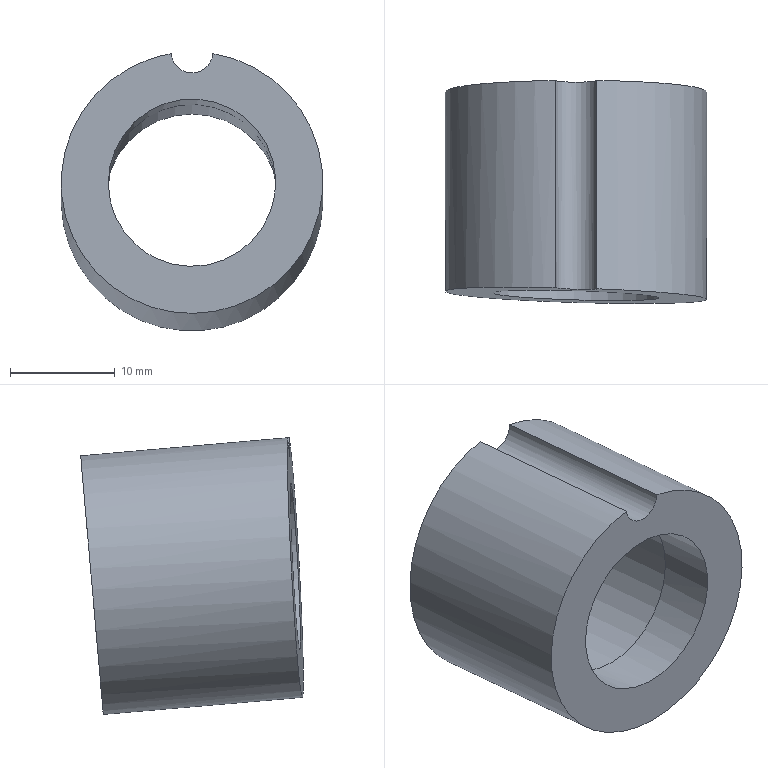Part | NX | features EKSD 25-20-16.00 2 | 1 solid | 7 faces | box 25 x 21.281 x 26.488 mm | volume 5318 mm3 | cylinder 4 | plane 3 | commonest cylinder face diameters 4 x1 16 x1 16.6 x1 25 x1
STEP:
#1=CARTESIAN_POINT('',(396.532,-42.364,-29.982));
#2=VERTEX_POINT('',#1);
#3=CARTESIAN_POINT('',(400.519,-42.364,-29.982));
#4=VERTEX_POINT('',#3);
#5=CARTESIAN_POINT('',(398.525,-42.35,-29.823));
#6=DIRECTION('',(0.,0.9962,-0.08716));
#7=DIRECTION('',(0.,0.08716,0.9962));
#8=AXIS2_PLACEMENT_3D('',#5,#6,#7);
#9=CIRCLE('',#8,2.);
#10=EDGE_CURVE('',#2,#4,#9,.F.);
#11=ORIENTED_EDGE('',*,*,#10,.T.);
#12=CARTESIAN_POINT('',(398.525,-43.44,-42.275));
#13=DIRECTION('',(0.,0.9962,-0.08716));
#14=DIRECTION('',(0.,0.08716,0.9962));
#15=AXIS2_PLACEMENT_3D('',#12,#13,#14);
#16=CIRCLE('',#15,12.5);
#17=EDGE_CURVE('',#2,#4,#16,.F.);
#18=ORIENTED_EDGE('',*,*,#17,.F.);
#19=EDGE_LOOP('',(#11,#18));
#20=FACE_BOUND('',#19,.T.);
#21=CARTESIAN_POINT('',(398.525,-42.717,-34.007));
#22=VERTEX_POINT('',#21);
#23=CARTESIAN_POINT('',(398.525,-43.44,-42.275));
#24=DIRECTION('',(0.,0.9962,-0.08716));
#25=DIRECTION('',(0.,0.08716,0.9962));
#26=AXIS2_PLACEMENT_3D('',#23,#24,#25);
#27=CIRCLE('',#26,8.3);
#28=EDGE_CURVE('',#22,#22,#27,.T.);
#29=ORIENTED_EDGE('',*,*,#28,.F.);
#30=EDGE_LOOP('',(#29));
#31=FACE_BOUND('',#30,.T.);
#32=CARTESIAN_POINT('',(398.525,-43.44,-42.275));
#33=DIRECTION('',(0.,0.9962,-0.08716));
#34=DIRECTION('',(0.,0.08716,0.9962));
#35=AXIS2_PLACEMENT_3D('',#32,#33,#34);
#36=PLANE('',#35);
#37=ADVANCED_FACE('',(#20,#31),#36,.T.);
#38=CARTESIAN_POINT('',(400.519,-62.276,-28.24));
#39=VERTEX_POINT('',#38);
#40=CARTESIAN_POINT('',(396.532,-62.155,-28.251));
#41=VERTEX_POINT('',#40);
#42=CARTESIAN_POINT('',(398.525,-62.207,-28.086));
#43=DIRECTION('',(0.03046,0.9981,-0.05344));
#44=DIRECTION('',(-0.6692,-0.01935,-0.7428));
#45=AXIS2_PLACEMENT_3D('',#42,#43,#44);
#46=ELLIPSE('',#45,2.002,2.);
#47=EDGE_CURVE('',#39,#41,#46,.T.);
#48=ORIENTED_EDGE('',*,*,#47,.T.);
#49=CARTESIAN_POINT('',(398.525,-62.876,-40.575));
#50=DIRECTION('',(0.03046,0.9981,-0.05344));
#51=DIRECTION('',(-0.6692,-0.01935,-0.7428));
#52=AXIS2_PLACEMENT_3D('',#49,#50,#51);
#53=ELLIPSE('',#52,12.513,12.5);
#54=EDGE_CURVE('',#39,#41,#53,.T.);
#55=ORIENTED_EDGE('',*,*,#54,.F.);
#56=EDGE_LOOP('',(#48,#55));
#57=FACE_BOUND('',#56,.T.);
#58=CARTESIAN_POINT('',(393.166,-63.031,-46.523));
#59=VERTEX_POINT('',#58);
#60=CARTESIAN_POINT('',(398.525,-62.876,-40.575));
#61=DIRECTION('',(0.03046,0.9981,-0.05344));
#62=DIRECTION('',(-0.6692,-0.01935,-0.7428));
#63=AXIS2_PLACEMENT_3D('',#60,#61,#62);
#64=ELLIPSE('',#63,8.008,8.);
#65=EDGE_CURVE('',#59,#59,#64,.F.);
#66=ORIENTED_EDGE('',*,*,#65,.F.);
#67=EDGE_LOOP('',(#66));
#68=FACE_BOUND('',#67,.T.);
#69=CARTESIAN_POINT('',(457.994,-68.531,-112.302));
#70=DIRECTION('',(0.03046,0.9981,-0.05344));
#71=DIRECTION('',(0.06614,0.05134,0.9965));
#72=AXIS2_PLACEMENT_3D('',#69,#70,#71);
#73=PLANE('',#72);
#74=ADVANCED_FACE('',(#57,#68),#73,.F.);
#75=CARTESIAN_POINT('',(400.519,-54.319,-28.936));
#76=DIRECTION('',(0.,0.9962,-0.08716));
#77=VECTOR('',#76,1000.);
#78=LINE('',#75,#77);
#79=EDGE_CURVE('',#39,#4,#78,.T.);
#80=ORIENTED_EDGE('',*,*,#79,.F.);
#81=ORIENTED_EDGE('',*,*,#54,.T.);
#82=CARTESIAN_POINT('',(396.532,-54.319,-28.936));
#83=DIRECTION('',(0.,0.9962,-0.08716));
#84=VECTOR('',#83,1000.);
#85=LINE('',#82,#84);
#86=EDGE_CURVE('',#2,#41,#85,.F.);
#87=ORIENTED_EDGE('',*,*,#86,.F.);
#88=ORIENTED_EDGE('',*,*,#17,.T.);
#89=EDGE_LOOP('',(#80,#81,#87,#88));
#90=FACE_BOUND('',#89,.T.);
#91=CARTESIAN_POINT('',(398.525,-65.356,-40.358));
#92=DIRECTION('',(0.,0.9962,-0.08716));
#93=DIRECTION('',(0.,0.08716,0.9962));
#94=AXIS2_PLACEMENT_3D('',#91,#92,#93);
#95=CYLINDRICAL_SURFACE('',#94,12.5);
#96=ADVANCED_FACE('',(#90),#95,.T.);
#97=CARTESIAN_POINT('',(398.525,-58.084,-49.025));
#98=VERTEX_POINT('',#97);
#99=CARTESIAN_POINT('',(398.525,-57.387,-41.055));
#100=DIRECTION('',(0.,-0.9962,0.08716));
#101=DIRECTION('',(0.,-0.08716,-0.9962));
#102=AXIS2_PLACEMENT_3D('',#99,#100,#101);
#103=CIRCLE('',#102,8.);
#104=EDGE_CURVE('',#98,#98,#103,.F.);
#105=ORIENTED_EDGE('',*,*,#104,.T.);
#106=EDGE_LOOP('',(#105));
#107=FACE_BOUND('',#106,.T.);
#108=ORIENTED_EDGE('',*,*,#65,.T.);
#109=EDGE_LOOP('',(#108));
#110=FACE_BOUND('',#109,.T.);
#111=CARTESIAN_POINT('',(398.525,-66.352,-40.271));
#112=DIRECTION('',(0.,0.9962,-0.08716));
#113=DIRECTION('',(0.,0.08716,0.9962));
#114=AXIS2_PLACEMENT_3D('',#111,#112,#113);
#115=CYLINDRICAL_SURFACE('',#114,8.);
#116=ADVANCED_FACE('',(#107,#110),#115,.F.);
#117=CARTESIAN_POINT('',(398.525,-56.663,-32.787));
#118=VERTEX_POINT('',#117);
#119=CARTESIAN_POINT('',(398.525,-57.387,-41.055));
#120=DIRECTION('',(0.,0.9962,-0.08716));
#121=DIRECTION('',(0.,0.08716,0.9962));
#122=AXIS2_PLACEMENT_3D('',#119,#120,#121);
#123=CIRCLE('',#122,8.3);
#124=EDGE_CURVE('',#118,#118,#123,.T.);
#125=ORIENTED_EDGE('',*,*,#124,.T.);
#126=EDGE_LOOP('',(#125));
#127=FACE_BOUND('',#126,.T.);
#128=ORIENTED_EDGE('',*,*,#104,.F.);
#129=EDGE_LOOP('',(#128));
#130=FACE_BOUND('',#129,.T.);
#131=CARTESIAN_POINT('',(398.525,-57.387,-41.055));
#132=DIRECTION('',(0.,-0.9962,0.08716));
#133=DIRECTION('',(0.,-0.08716,-0.9962));
#134=AXIS2_PLACEMENT_3D('',#131,#132,#133);
#135=PLANE('',#134);
#136=ADVANCED_FACE('',(#127,#130),#135,.F.);
#137=ORIENTED_EDGE('',*,*,#28,.T.);
#138=EDGE_LOOP('',(#137));
#139=FACE_BOUND('',#138,.T.);
#140=ORIENTED_EDGE('',*,*,#124,.F.);
#141=EDGE_LOOP('',(#140));
#142=FACE_BOUND('',#141,.T.);
#143=CARTESIAN_POINT('',(398.525,-57.387,-41.055));
#144=DIRECTION('',(0.,0.9962,-0.08716));
#145=DIRECTION('',(0.,0.08716,0.9962));
#146=AXIS2_PLACEMENT_3D('',#143,#144,#145);
#147=CYLINDRICAL_SURFACE('',#146,8.3);
#148=ADVANCED_FACE('',(#139,#142),#147,.F.);
#149=ORIENTED_EDGE('',*,*,#79,.T.);
#150=ORIENTED_EDGE('',*,*,#10,.F.);
#151=ORIENTED_EDGE('',*,*,#86,.T.);
#152=ORIENTED_EDGE('',*,*,#47,.F.);
#153=EDGE_LOOP('',(#149,#150,#151,#152));
#154=FACE_BOUND('',#153,.T.);
#155=CARTESIAN_POINT('',(398.525,-64.267,-27.905));
#156=DIRECTION('',(0.,0.9962,-0.08716));
#157=DIRECTION('',(0.,0.08716,0.9962));
#158=AXIS2_PLACEMENT_3D('',#155,#156,#157);
#159=CYLINDRICAL_SURFACE('',#158,2.);
#160=ADVANCED_FACE('',(#154),#159,.F.);
#161=CLOSED_SHELL('',(#37,#74,#96,#116,#136,#148,#160));
#162=MANIFOLD_SOLID_BREP('',#161);
#163=(LENGTH_UNIT()NAMED_UNIT(*)SI_UNIT(.MILLI.,.METRE.));
#164=UNCERTAINTY_MEASURE_WITH_UNIT(LENGTH_MEASURE(0.00001),#163,'','');
#165=(NAMED_UNIT(*)PLANE_ANGLE_UNIT()SI_UNIT($,.RADIAN.));
#166=(NAMED_UNIT(*)SI_UNIT($,.STERADIAN.)SOLID_ANGLE_UNIT());
#167=(GEOMETRIC_REPRESENTATION_CONTEXT(3)GLOBAL_UNCERTAINTY_ASSIGNED_CONTEXT((#164))GLOBAL_UNIT_ASSIGNED_CONTEXT((#163,#165,#166))REPRESENTATION_CONTEXT('',''));
#168=ADVANCED_BREP_SHAPE_REPRESENTATION('',(#162),#167);